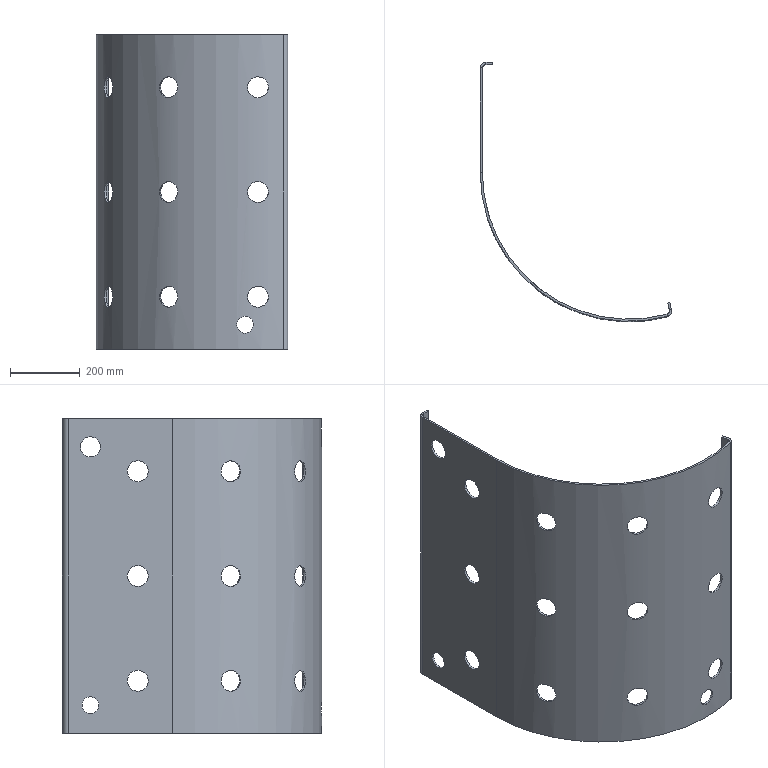Part | SolidWorks | features EdgeFlange 2, ICE 2, RevCut 2, CirPattern 1, FlatPattern 1, LPattern 1, SMBaseFlange 1, SheetMetal 1 | 1 solid | 56 faces | box 548.116 x 742 x 900 mm | volume 6001500 mm3 | cylinder 36 | plane 20 | commonest cylinder face diameters 60 x24 48 x4 20 x2 32 x2 57.542 x2 840 x1